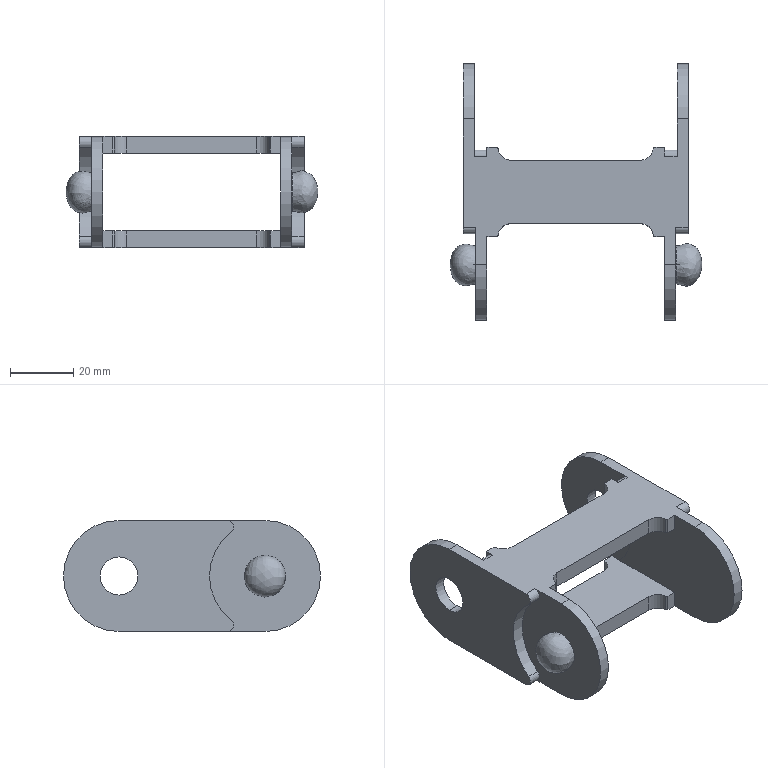Part | STEP file | TWH25-C57-R75-CONNECTION | 2 solids | 77 faces | box 79.373 x 81 x 35 mm | volume 33777 mm3 | cylinder 40 | plane 30 | spline 5 | torus 2 | commonest cylinder face diameters 1 x8 4 x8 8 x8 12 x8 35 x8